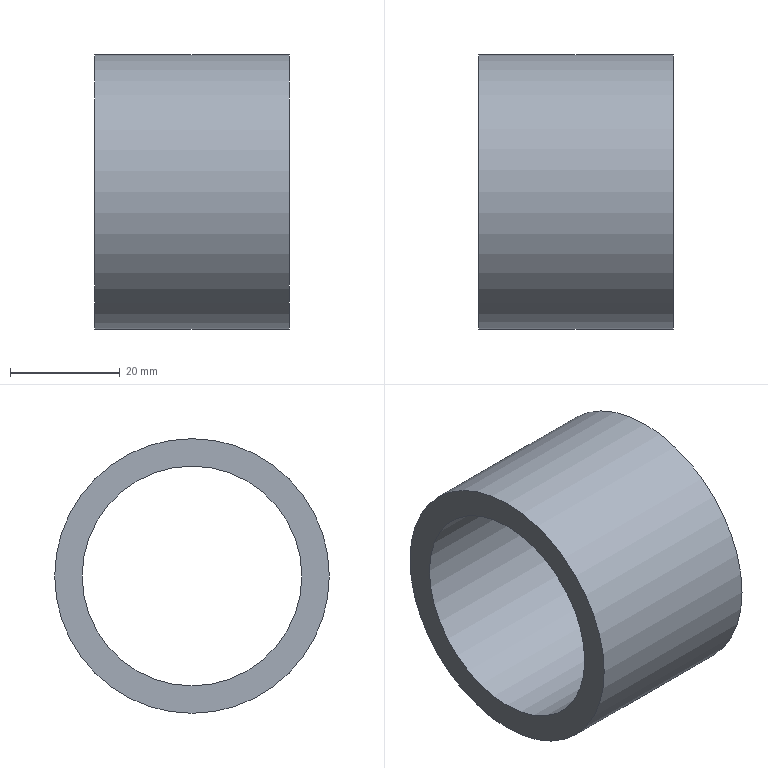Part | NX | features DATUM_CSYS 2, EXTRUDE 1, SKETCH 1 | 1 solid | 4 faces | box 35.5 x 50 x 50 mm | volume 25093 mm3 | cylinder 2 | plane 2 | commonest cylinder face diameters 40 x1 50 x1
STEP:
#1=CARTESIAN_POINT('',(35.5,25.,0.));
#2=VERTEX_POINT('',#1);
#3=CARTESIAN_POINT('',(35.5,0.,0.));
#4=DIRECTION('',(1.,0.,0.));
#5=DIRECTION('',(0.,1.,0.));
#6=AXIS2_PLACEMENT_3D('',#3,#4,#5);
#7=CIRCLE('',#6,25.);
#8=EDGE_CURVE('',#2,#2,#7,.T.);
#9=ORIENTED_EDGE('',*,*,#8,.F.);
#10=EDGE_LOOP('',(#9));
#11=FACE_BOUND('',#10,.T.);
#12=CARTESIAN_POINT('',(0.,25.,0.));
#13=VERTEX_POINT('',#12);
#14=CARTESIAN_POINT('',(0.,0.,0.));
#15=DIRECTION('',(1.,0.,0.));
#16=DIRECTION('',(0.,1.,0.));
#17=AXIS2_PLACEMENT_3D('',#14,#15,#16);
#18=CIRCLE('',#17,25.);
#19=EDGE_CURVE('',#13,#13,#18,.T.);
#20=ORIENTED_EDGE('',*,*,#19,.T.);
#21=EDGE_LOOP('',(#20));
#22=FACE_BOUND('',#21,.T.);
#23=CARTESIAN_POINT('',(35.5,0.,0.));
#24=DIRECTION('',(-1.,0.,0.));
#25=DIRECTION('',(0.,0.,1.));
#26=AXIS2_PLACEMENT_3D('',#23,#24,#25);
#27=CYLINDRICAL_SURFACE('',#26,25.);
#28=ADVANCED_FACE('',(#11,#22),#27,.T.);
#29=CARTESIAN_POINT('',(35.5,20.,0.));
#30=VERTEX_POINT('',#29);
#31=CARTESIAN_POINT('',(35.5,0.,0.));
#32=DIRECTION('',(1.,0.,0.));
#33=DIRECTION('',(0.,1.,0.));
#34=AXIS2_PLACEMENT_3D('',#31,#32,#33);
#35=CIRCLE('',#34,20.);
#36=EDGE_CURVE('',#30,#30,#35,.T.);
#37=ORIENTED_EDGE('',*,*,#36,.T.);
#38=EDGE_LOOP('',(#37));
#39=FACE_BOUND('',#38,.T.);
#40=CARTESIAN_POINT('',(0.,20.,0.));
#41=VERTEX_POINT('',#40);
#42=CARTESIAN_POINT('',(0.,0.,0.));
#43=DIRECTION('',(1.,0.,0.));
#44=DIRECTION('',(0.,1.,0.));
#45=AXIS2_PLACEMENT_3D('',#42,#43,#44);
#46=CIRCLE('',#45,20.);
#47=EDGE_CURVE('',#41,#41,#46,.T.);
#48=ORIENTED_EDGE('',*,*,#47,.F.);
#49=EDGE_LOOP('',(#48));
#50=FACE_BOUND('',#49,.T.);
#51=CARTESIAN_POINT('',(35.5,0.,0.));
#52=DIRECTION('',(-1.,0.,0.));
#53=DIRECTION('',(0.,0.,1.));
#54=AXIS2_PLACEMENT_3D('',#51,#52,#53);
#55=CYLINDRICAL_SURFACE('',#54,20.);
#56=ADVANCED_FACE('',(#39,#50),#55,.F.);
#57=ORIENTED_EDGE('',*,*,#8,.T.);
#58=EDGE_LOOP('',(#57));
#59=FACE_BOUND('',#58,.T.);
#60=ORIENTED_EDGE('',*,*,#36,.F.);
#61=EDGE_LOOP('',(#60));
#62=FACE_BOUND('',#61,.T.);
#63=CARTESIAN_POINT('',(35.5,0.,0.));
#64=DIRECTION('',(1.,0.,0.));
#65=DIRECTION('',(0.,0.,-1.));
#66=AXIS2_PLACEMENT_3D('',#63,#64,#65);
#67=PLANE('',#66);
#68=ADVANCED_FACE('',(#59,#62),#67,.T.);
#69=ORIENTED_EDGE('',*,*,#19,.F.);
#70=EDGE_LOOP('',(#69));
#71=FACE_BOUND('',#70,.T.);
#72=ORIENTED_EDGE('',*,*,#47,.T.);
#73=EDGE_LOOP('',(#72));
#74=FACE_BOUND('',#73,.T.);
#75=CARTESIAN_POINT('',(0.,0.,0.));
#76=DIRECTION('',(1.,0.,0.));
#77=DIRECTION('',(0.,0.,-1.));
#78=AXIS2_PLACEMENT_3D('',#75,#76,#77);
#79=PLANE('',#78);
#80=ADVANCED_FACE('',(#71,#74),#79,.F.);
#81=CLOSED_SHELL('',(#28,#56,#68,#80));
#82=MANIFOLD_SOLID_BREP('',#81);
#83=(LENGTH_UNIT()NAMED_UNIT(*)SI_UNIT(.MILLI.,.METRE.));
#84=UNCERTAINTY_MEASURE_WITH_UNIT(LENGTH_MEASURE(0.00001),#83,'','');
#85=(NAMED_UNIT(*)PLANE_ANGLE_UNIT()SI_UNIT($,.RADIAN.));
#86=(NAMED_UNIT(*)SI_UNIT($,.STERADIAN.)SOLID_ANGLE_UNIT());
#87=(GEOMETRIC_REPRESENTATION_CONTEXT(3)GLOBAL_UNCERTAINTY_ASSIGNED_CONTEXT((#84))GLOBAL_UNIT_ASSIGNED_CONTEXT((#83,#85,#86))REPRESENTATION_CONTEXT('',''));
#88=ADVANCED_BREP_SHAPE_REPRESENTATION('',(#82),#87);